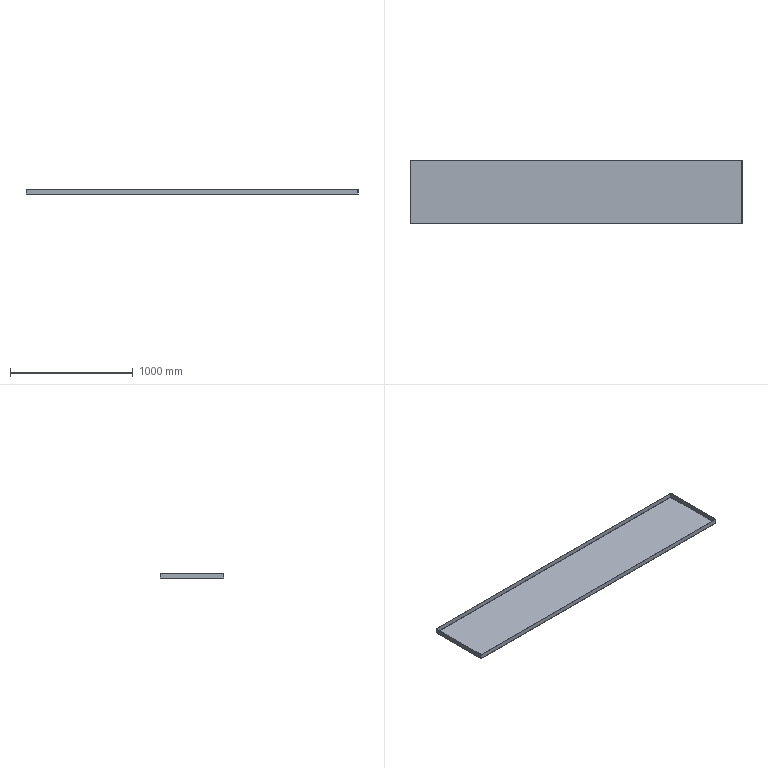Part | SolidWorks | features EdgeFlange 1, FlatPattern 1, SMBaseFlange 1, SheetMetal 1 | 1 solid | 38 faces | box 2700 x 518 x 40 mm | volume 3275069 mm3 | plane 22 | spline 8 | cylinder 8 | commonest cylinder face diameters 1.473 x4 5.473 x4
STEP:
#1=CARTESIAN_POINT('',(1347.263,256.263,-2.));
#2=VERTEX_POINT('',#1);
#3=CARTESIAN_POINT('',(1347.263,-256.263,-2.));
#4=VERTEX_POINT('',#3);
#5=CARTESIAN_POINT('',(1347.263,256.293,-2.));
#6=DIRECTION('',(0.,-1.,0.));
#7=VECTOR('',#6,1000.);
#8=LINE('',#5,#7);
#9=EDGE_CURVE('',#2,#4,#8,.T.);
#10=ORIENTED_EDGE('',*,*,#9,.T.);
#11=CARTESIAN_POINT('',(-1347.263,-256.263,-2.));
#12=VERTEX_POINT('',#11);
#13=CARTESIAN_POINT('',(1347.293,-256.263,-2.));
#14=DIRECTION('',(-1.,0.,0.));
#15=VECTOR('',#14,1000.);
#16=LINE('',#13,#15);
#17=EDGE_CURVE('',#4,#12,#16,.T.);
#18=ORIENTED_EDGE('',*,*,#17,.T.);
#19=CARTESIAN_POINT('',(-1347.263,256.263,-2.));
#20=VERTEX_POINT('',#19);
#21=CARTESIAN_POINT('',(-1347.263,-256.293,-2.));
#22=DIRECTION('',(0.,1.,0.));
#23=VECTOR('',#22,1000.);
#24=LINE('',#21,#23);
#25=EDGE_CURVE('',#12,#20,#24,.T.);
#26=ORIENTED_EDGE('',*,*,#25,.T.);
#27=CARTESIAN_POINT('',(-1347.293,256.263,-2.));
#28=DIRECTION('',(1.,0.,0.));
#29=VECTOR('',#28,1000.);
#30=LINE('',#27,#29);
#31=EDGE_CURVE('',#20,#2,#30,.T.);
#32=ORIENTED_EDGE('',*,*,#31,.T.);
#33=EDGE_LOOP('',(#10,#18,#26,#32));
#34=FACE_OUTER_BOUND('',#33,.T.);
#35=CARTESIAN_POINT('',(0.,0.,-2.));
#36=DIRECTION('',(0.,0.,-1.));
#37=DIRECTION('',(-1.,0.,0.));
#38=AXIS2_PLACEMENT_3D('',#35,#36,#37);
#39=PLANE('',#38);
#40=ADVANCED_FACE('',(#34),#39,.T.);
#41=CARTESIAN_POINT('',(1347.263,-256.263,0.));
#42=VERTEX_POINT('',#41);
#43=CARTESIAN_POINT('',(-1347.263,-256.263,0.));
#44=VERTEX_POINT('',#43);
#45=CARTESIAN_POINT('',(1347.293,-256.263,0.));
#46=DIRECTION('',(-1.,0.,0.));
#47=VECTOR('',#46,1000.);
#48=LINE('',#45,#47);
#49=EDGE_CURVE('',#42,#44,#48,.T.);
#50=ORIENTED_EDGE('',*,*,#49,.F.);
#51=CARTESIAN_POINT('',(1347.263,256.263,0.));
#52=VERTEX_POINT('',#51);
#53=CARTESIAN_POINT('',(1347.263,256.293,0.));
#54=DIRECTION('',(0.,-1.,0.));
#55=VECTOR('',#54,1000.);
#56=LINE('',#53,#55);
#57=EDGE_CURVE('',#52,#42,#56,.T.);
#58=ORIENTED_EDGE('',*,*,#57,.F.);
#59=CARTESIAN_POINT('',(-1347.263,256.263,0.));
#60=VERTEX_POINT('',#59);
#61=CARTESIAN_POINT('',(-1347.293,256.263,0.));
#62=DIRECTION('',(1.,0.,0.));
#63=VECTOR('',#62,1000.);
#64=LINE('',#61,#63);
#65=EDGE_CURVE('',#60,#52,#64,.T.);
#66=ORIENTED_EDGE('',*,*,#65,.F.);
#67=CARTESIAN_POINT('',(-1347.263,-256.293,0.));
#68=DIRECTION('',(0.,1.,0.));
#69=VECTOR('',#68,1000.);
#70=LINE('',#67,#69);
#71=EDGE_CURVE('',#44,#60,#70,.T.);
#72=ORIENTED_EDGE('',*,*,#71,.F.);
#73=EDGE_LOOP('',(#50,#58,#66,#72));
#74=FACE_OUTER_BOUND('',#73,.T.);
#75=CARTESIAN_POINT('',(0.,0.,0.));
#76=DIRECTION('',(0.,0.,-1.));
#77=DIRECTION('',(-1.,0.,0.));
#78=AXIS2_PLACEMENT_3D('',#75,#76,#77);
#79=PLANE('',#78);
#80=ADVANCED_FACE('',(#74),#79,.F.);
#81=CARTESIAN_POINT('',(1347.293,259.,0.7366));
#82=VERTEX_POINT('',#81);
#83=CARTESIAN_POINT('',(1347.293,257.,0.7366));
#84=VERTEX_POINT('',#83);
#85=CARTESIAN_POINT('',(1347.293,257.,0.7366));
#86=DIRECTION('',(0.,-1.,0.));
#87=VECTOR('',#86,1000.);
#88=LINE('',#85,#87);
#89=EDGE_CURVE('',#82,#84,#88,.T.);
#90=ORIENTED_EDGE('',*,*,#89,.T.);
#91=CARTESIAN_POINT('',(1347.263,256.263,0.));
#92=CARTESIAN_POINT('',(1347.268,256.456,0.));
#93=CARTESIAN_POINT('',(1347.273,256.648,0.07939));
#94=CARTESIAN_POINT('',(1347.283,256.921,0.3521));
#95=CARTESIAN_POINT('',(1347.288,257.,0.5438));
#96=CARTESIAN_POINT('',(1347.293,257.,0.7366));
#97=B_SPLINE_CURVE_WITH_KNOTS('',3,(#91,#92,#93,#94,#95,#96),.UNSPECIFIED.,.F.,.F.,(4,2,4),(0.,0.5,1.),.UNSPECIFIED.);
#98=EDGE_CURVE('',#52,#84,#97,.T.);
#99=ORIENTED_EDGE('',*,*,#98,.F.);
#100=CARTESIAN_POINT('',(1347.263,256.263,0.));
#101=DIRECTION('',(0.,0.,-1.));
#102=VECTOR('',#101,1000.);
#103=LINE('',#100,#102);
#104=EDGE_CURVE('',#52,#2,#103,.T.);
#105=ORIENTED_EDGE('',*,*,#104,.T.);
#106=CARTESIAN_POINT('',(1347.263,256.263,-2.));
#107=CARTESIAN_POINT('',(1347.266,256.622,-2.));
#108=CARTESIAN_POINT('',(1347.268,256.98,-1.929));
#109=CARTESIAN_POINT('',(1347.273,257.642,-1.655));
#110=CARTESIAN_POINT('',(1347.276,257.945,-1.452));
#111=CARTESIAN_POINT('',(1347.281,258.452,-0.9452));
#112=CARTESIAN_POINT('',(1347.283,258.655,-0.6416));
#113=CARTESIAN_POINT('',(1347.288,258.929,0.0203));
#114=CARTESIAN_POINT('',(1347.29,259.,0.3784));
#115=CARTESIAN_POINT('',(1347.293,259.,0.7366));
#116=B_SPLINE_CURVE_WITH_KNOTS('',3,(#106,#107,#108,#109,#110,#111,#112,#113,#114,#115),.UNSPECIFIED.,.F.,.F.,(4,2,2,2,4),(0.,0.25,0.5,0.75,1.),.UNSPECIFIED.);
#117=EDGE_CURVE('',#2,#82,#116,.T.);
#118=ORIENTED_EDGE('',*,*,#117,.T.);
#119=EDGE_LOOP('',(#90,#99,#105,#118));
#120=FACE_OUTER_BOUND('',#119,.T.);
#121=CARTESIAN_POINT('',(1347.263,256.263,-2.02));
#122=CARTESIAN_POINT('',(1347.266,256.624,-2.02));
#123=CARTESIAN_POINT('',(1347.268,256.985,-1.948));
#124=CARTESIAN_POINT('',(1347.273,257.652,-1.672));
#125=CARTESIAN_POINT('',(1347.276,257.957,-1.468));
#126=CARTESIAN_POINT('',(1347.281,258.468,-0.9575));
#127=CARTESIAN_POINT('',(1347.283,258.672,-0.6517));
#128=CARTESIAN_POINT('',(1347.288,258.948,0.01507));
#129=CARTESIAN_POINT('',(1347.29,259.02,0.3757));
#130=CARTESIAN_POINT('',(1347.293,259.02,0.7366));
#131=CARTESIAN_POINT('',(1347.263,256.263,-2.));
#132=CARTESIAN_POINT('',(1347.266,256.622,-2.));
#133=CARTESIAN_POINT('',(1347.268,256.98,-1.929));
#134=CARTESIAN_POINT('',(1347.273,257.642,-1.655));
#135=CARTESIAN_POINT('',(1347.276,257.945,-1.452));
#136=CARTESIAN_POINT('',(1347.281,258.452,-0.9452));
#137=CARTESIAN_POINT('',(1347.283,258.655,-0.6416));
#138=CARTESIAN_POINT('',(1347.288,258.929,0.0203));
#139=CARTESIAN_POINT('',(1347.29,259.,0.3783));
#140=CARTESIAN_POINT('',(1347.293,259.,0.7366));
#141=CARTESIAN_POINT('',(1347.263,256.263,0.));
#142=CARTESIAN_POINT('',(1347.266,256.36,0.));
#143=CARTESIAN_POINT('',(1347.268,256.456,0.01917));
#144=CARTESIAN_POINT('',(1347.273,256.634,0.09297));
#145=CARTESIAN_POINT('',(1347.276,256.716,0.1476));
#146=CARTESIAN_POINT('',(1347.281,256.852,0.2839));
#147=CARTESIAN_POINT('',(1347.283,256.907,0.3656));
#148=CARTESIAN_POINT('',(1347.288,256.981,0.5438));
#149=CARTESIAN_POINT('',(1347.29,257.,0.6402));
#150=CARTESIAN_POINT('',(1347.293,257.,0.7366));
#151=CARTESIAN_POINT('',(1347.263,256.263,0.0202));
#152=CARTESIAN_POINT('',(1347.266,256.357,0.0202));
#153=CARTESIAN_POINT('',(1347.268,256.451,0.03885));
#154=CARTESIAN_POINT('',(1347.273,256.624,0.1106));
#155=CARTESIAN_POINT('',(1347.276,256.704,0.1637));
#156=CARTESIAN_POINT('',(1347.281,256.836,0.2963));
#157=CARTESIAN_POINT('',(1347.283,256.889,0.3758));
#158=CARTESIAN_POINT('',(1347.288,256.961,0.5491));
#159=CARTESIAN_POINT('',(1347.29,256.98,0.6428));
#160=CARTESIAN_POINT('',(1347.293,256.98,0.7366));
#161=B_SPLINE_SURFACE_WITH_KNOTS('',1,3,((#121,#122,#123,#124,#125,#126,#127,#128,#129,#130),(#131,#132,#133,#134,#135,#136,#137,#138,#139,#140),(#141,#142,#143,#144,#145,#146,#147,#148,#149,#150),(#151,#152,#153,#154,#155,#156,#157,#158,#159,#160)),.UNSPECIFIED.,.F.,.F.,.F.,(2,1,1,2),(4,2,2,2,4),(-0.01,0.,1.,1.01),(0.,0.25,0.5,0.75,1.),.UNSPECIFIED.);
#162=ADVANCED_FACE('',(#120),#161,.F.);
#163=CARTESIAN_POINT('',(-1347.293,257.,0.7366));
#164=VERTEX_POINT('',#163);
#165=CARTESIAN_POINT('',(-1347.293,257.,0.7366));
#166=CARTESIAN_POINT('',(-1347.288,257.,0.5438));
#167=CARTESIAN_POINT('',(-1347.283,256.921,0.3521));
#168=CARTESIAN_POINT('',(-1347.273,256.648,0.07939));
#169=CARTESIAN_POINT('',(-1347.268,256.456,0.));
#170=CARTESIAN_POINT('',(-1347.263,256.263,0.));
#171=B_SPLINE_CURVE_WITH_KNOTS('',3,(#165,#166,#167,#168,#169,#170),.UNSPECIFIED.,.F.,.F.,(4,2,4),(0.,0.5,1.),.UNSPECIFIED.);
#172=EDGE_CURVE('',#164,#60,#171,.T.);
#173=ORIENTED_EDGE('',*,*,#172,.F.);
#174=CARTESIAN_POINT('',(-1347.293,259.,0.7366));
#175=VERTEX_POINT('',#174);
#176=CARTESIAN_POINT('',(-1347.293,257.,0.7366));
#177=DIRECTION('',(0.,-1.,0.));
#178=VECTOR('',#177,1000.);
#179=LINE('',#176,#178);
#180=EDGE_CURVE('',#175,#164,#179,.T.);
#181=ORIENTED_EDGE('',*,*,#180,.F.);
#182=CARTESIAN_POINT('',(-1347.293,259.,0.7366));
#183=CARTESIAN_POINT('',(-1347.29,259.,0.3784));
#184=CARTESIAN_POINT('',(-1347.288,258.929,0.0203));
#185=CARTESIAN_POINT('',(-1347.283,258.655,-0.6416));
#186=CARTESIAN_POINT('',(-1347.281,258.452,-0.9452));
#187=CARTESIAN_POINT('',(-1347.276,257.945,-1.452));
#188=CARTESIAN_POINT('',(-1347.273,257.642,-1.655));
#189=CARTESIAN_POINT('',(-1347.268,256.98,-1.929));
#190=CARTESIAN_POINT('',(-1347.266,256.622,-2.));
#191=CARTESIAN_POINT('',(-1347.263,256.263,-2.));
#192=B_SPLINE_CURVE_WITH_KNOTS('',3,(#182,#183,#184,#185,#186,#187,#188,#189,#190,#191),.UNSPECIFIED.,.F.,.F.,(4,2,2,2,4),(0.,0.25,0.5,0.75,1.),.UNSPECIFIED.);
#193=EDGE_CURVE('',#175,#20,#192,.T.);
#194=ORIENTED_EDGE('',*,*,#193,.T.);
#195=CARTESIAN_POINT('',(-1347.263,256.263,0.));
#196=DIRECTION('',(0.,0.,-1.));
#197=VECTOR('',#196,1000.);
#198=LINE('',#195,#197);
#199=EDGE_CURVE('',#60,#20,#198,.T.);
#200=ORIENTED_EDGE('',*,*,#199,.F.);
#201=EDGE_LOOP('',(#173,#181,#194,#200));
#202=FACE_OUTER_BOUND('',#201,.T.);
#203=CARTESIAN_POINT('',(-1347.293,259.02,0.7366));
#204=CARTESIAN_POINT('',(-1347.29,259.02,0.3757));
#205=CARTESIAN_POINT('',(-1347.288,258.948,0.01507));
#206=CARTESIAN_POINT('',(-1347.283,258.672,-0.6517));
#207=CARTESIAN_POINT('',(-1347.281,258.468,-0.9575));
#208=CARTESIAN_POINT('',(-1347.276,257.957,-1.468));
#209=CARTESIAN_POINT('',(-1347.273,257.652,-1.672));
#210=CARTESIAN_POINT('',(-1347.268,256.985,-1.948));
#211=CARTESIAN_POINT('',(-1347.266,256.624,-2.02));
#212=CARTESIAN_POINT('',(-1347.263,256.263,-2.02));
#213=CARTESIAN_POINT('',(-1347.293,259.,0.7366));
#214=CARTESIAN_POINT('',(-1347.29,259.,0.3783));
#215=CARTESIAN_POINT('',(-1347.288,258.929,0.0203));
#216=CARTESIAN_POINT('',(-1347.283,258.655,-0.6416));
#217=CARTESIAN_POINT('',(-1347.281,258.452,-0.9452));
#218=CARTESIAN_POINT('',(-1347.276,257.945,-1.452));
#219=CARTESIAN_POINT('',(-1347.273,257.642,-1.655));
#220=CARTESIAN_POINT('',(-1347.268,256.98,-1.929));
#221=CARTESIAN_POINT('',(-1347.266,256.622,-2.));
#222=CARTESIAN_POINT('',(-1347.263,256.263,-2.));
#223=CARTESIAN_POINT('',(-1347.293,257.,0.7366));
#224=CARTESIAN_POINT('',(-1347.29,257.,0.6402));
#225=CARTESIAN_POINT('',(-1347.288,256.981,0.5438));
#226=CARTESIAN_POINT('',(-1347.283,256.907,0.3656));
#227=CARTESIAN_POINT('',(-1347.281,256.852,0.2839));
#228=CARTESIAN_POINT('',(-1347.276,256.716,0.1476));
#229=CARTESIAN_POINT('',(-1347.273,256.634,0.09297));
#230=CARTESIAN_POINT('',(-1347.268,256.456,0.01917));
#231=CARTESIAN_POINT('',(-1347.266,256.36,0.));
#232=CARTESIAN_POINT('',(-1347.263,256.263,0.));
#233=CARTESIAN_POINT('',(-1347.293,256.98,0.7366));
#234=CARTESIAN_POINT('',(-1347.29,256.98,0.6428));
#235=CARTESIAN_POINT('',(-1347.288,256.961,0.5491));
#236=CARTESIAN_POINT('',(-1347.283,256.889,0.3758));
#237=CARTESIAN_POINT('',(-1347.281,256.836,0.2963));
#238=CARTESIAN_POINT('',(-1347.276,256.704,0.1637));
#239=CARTESIAN_POINT('',(-1347.273,256.624,0.1106));
#240=CARTESIAN_POINT('',(-1347.268,256.451,0.03885));
#241=CARTESIAN_POINT('',(-1347.266,256.357,0.0202));
#242=CARTESIAN_POINT('',(-1347.263,256.263,0.0202));
#243=B_SPLINE_SURFACE_WITH_KNOTS('',1,3,((#203,#204,#205,#206,#207,#208,#209,#210,#211,#212),(#213,#214,#215,#216,#217,#218,#219,#220,#221,#222),(#223,#224,#225,#226,#227,#228,#229,#230,#231,#232),(#233,#234,#235,#236,#237,#238,#239,#240,#241,#242)),.UNSPECIFIED.,.F.,.F.,.F.,(2,1,1,2),(4,2,2,2,4),(-0.01,0.,1.,1.01),(0.,0.25,0.5,0.75,1.),.UNSPECIFIED.);
#244=ADVANCED_FACE('',(#202),#243,.F.);
#245=ORIENTED_EDGE('',*,*,#31,.F.);
#246=ORIENTED_EDGE('',*,*,#193,.F.);
#247=CARTESIAN_POINT('',(0.,259.,0.7366));
#248=DIRECTION('',(-1.,0.,0.));
#249=VECTOR('',#248,1000.);
#250=LINE('',#247,#249);
#251=EDGE_CURVE('',#82,#175,#250,.T.);
#252=ORIENTED_EDGE('',*,*,#251,.F.);
#253=ORIENTED_EDGE('',*,*,#117,.F.);
#254=EDGE_LOOP('',(#245,#246,#252,#253));
#255=FACE_OUTER_BOUND('',#254,.T.);
#256=CARTESIAN_POINT('',(-1347.293,256.263,0.7366));
#257=DIRECTION('',(-1.,0.,0.));
#258=DIRECTION('',(0.,1.,0.));
#259=AXIS2_PLACEMENT_3D('',#256,#257,#258);
#260=CYLINDRICAL_SURFACE('',#259,2.737);
#261=ADVANCED_FACE('',(#255),#260,.T.);
#262=ORIENTED_EDGE('',*,*,#65,.T.);
#263=ORIENTED_EDGE('',*,*,#98,.T.);
#264=CARTESIAN_POINT('',(1350.,257.,0.7366));
#265=DIRECTION('',(-1.,0.,0.));
#266=VECTOR('',#265,1000.);
#267=LINE('',#264,#266);
#268=EDGE_CURVE('',#84,#164,#267,.T.);
#269=ORIENTED_EDGE('',*,*,#268,.T.);
#270=ORIENTED_EDGE('',*,*,#172,.T.);
#271=EDGE_LOOP('',(#262,#263,#269,#270));
#272=FACE_OUTER_BOUND('',#271,.T.);
#273=CARTESIAN_POINT('',(-1347.293,256.263,0.7366));
#274=DIRECTION('',(-1.,0.,0.));
#275=DIRECTION('',(0.,1.,0.));
#276=AXIS2_PLACEMENT_3D('',#273,#274,#275);
#277=CYLINDRICAL_SURFACE('',#276,0.7366);
#278=ADVANCED_FACE('',(#272),#277,.F.);
#279=CARTESIAN_POINT('',(1347.293,257.,38.));
#280=VERTEX_POINT('',#279);
#281=CARTESIAN_POINT('',(1347.293,259.,38.));
#282=VERTEX_POINT('',#281);
#283=CARTESIAN_POINT('',(1347.293,259.,38.));
#284=DIRECTION('',(0.,1.,0.));
#285=VECTOR('',#284,1000.);
#286=LINE('',#283,#285);
#287=EDGE_CURVE('',#280,#282,#286,.T.);
#288=ORIENTED_EDGE('',*,*,#287,.F.);
#289=CARTESIAN_POINT('',(1347.293,257.,0.));
#290=DIRECTION('',(0.,0.,1.));
#291=VECTOR('',#290,1000.);
#292=LINE('',#289,#291);
#293=EDGE_CURVE('',#84,#280,#292,.T.);
#294=ORIENTED_EDGE('',*,*,#293,.F.);
#295=ORIENTED_EDGE('',*,*,#89,.F.);
#296=CARTESIAN_POINT('',(1347.293,259.,0.));
#297=DIRECTION('',(0.,0.,-1.));
#298=VECTOR('',#297,1000.);
#299=LINE('',#296,#298);
#300=EDGE_CURVE('',#282,#82,#299,.T.);
#301=ORIENTED_EDGE('',*,*,#300,.F.);
#302=EDGE_LOOP('',(#288,#294,#295,#301));
#303=FACE_OUTER_BOUND('',#302,.T.);
#304=CARTESIAN_POINT('',(1347.293,257.,0.));
#305=DIRECTION('',(1.,0.,0.));
#306=DIRECTION('',(0.,0.,-1.));
#307=AXIS2_PLACEMENT_3D('',#304,#305,#306);
#308=PLANE('',#307);
#309=ADVANCED_FACE('',(#303),#308,.T.);
#310=CARTESIAN_POINT('',(-1347.293,259.,38.));
#311=VERTEX_POINT('',#310);
#312=CARTESIAN_POINT('',(-1347.293,259.,0.));
#313=DIRECTION('',(0.,0.,-1.));
#314=VECTOR('',#313,1000.);
#315=LINE('',#312,#314);
#316=EDGE_CURVE('',#311,#175,#315,.T.);
#317=ORIENTED_EDGE('',*,*,#316,.F.);
#318=CARTESIAN_POINT('',(-1350.,259.,38.));
#319=DIRECTION('',(-1.,0.,0.));
#320=VECTOR('',#319,1000.);
#321=LINE('',#318,#320);
#322=EDGE_CURVE('',#282,#311,#321,.T.);
#323=ORIENTED_EDGE('',*,*,#322,.F.);
#324=ORIENTED_EDGE('',*,*,#300,.T.);
#325=ORIENTED_EDGE('',*,*,#251,.T.);
#326=EDGE_LOOP('',(#317,#323,#324,#325));
#327=FACE_OUTER_BOUND('',#326,.T.);
#328=CARTESIAN_POINT('',(0.,259.,0.));
#329=DIRECTION('',(0.,1.,0.));
#330=DIRECTION('',(0.,0.,1.));
#331=AXIS2_PLACEMENT_3D('',#328,#329,#330);
#332=PLANE('',#331);
#333=ADVANCED_FACE('',(#327),#332,.T.);
#334=CARTESIAN_POINT('',(-1347.293,257.,38.));
#335=VERTEX_POINT('',#334);
#336=CARTESIAN_POINT('',(0.,257.,38.));
#337=DIRECTION('',(-1.,0.,0.));
#338=VECTOR('',#337,1000.);
#339=LINE('',#336,#338);
#340=EDGE_CURVE('',#280,#335,#339,.T.);
#341=ORIENTED_EDGE('',*,*,#340,.T.);
#342=CARTESIAN_POINT('',(-1347.293,257.,0.));
#343=DIRECTION('',(0.,0.,1.));
#344=VECTOR('',#343,1000.);
#345=LINE('',#342,#344);
#346=EDGE_CURVE('',#164,#335,#345,.T.);
#347=ORIENTED_EDGE('',*,*,#346,.F.);
#348=ORIENTED_EDGE('',*,*,#268,.F.);
#349=ORIENTED_EDGE('',*,*,#293,.T.);
#350=EDGE_LOOP('',(#341,#347,#348,#349));
#351=FACE_OUTER_BOUND('',#350,.T.);
#352=CARTESIAN_POINT('',(0.,257.,0.));
#353=DIRECTION('',(0.,1.,0.));
#354=DIRECTION('',(0.,0.,1.));
#355=AXIS2_PLACEMENT_3D('',#352,#353,#354);
#356=PLANE('',#355);
#357=ADVANCED_FACE('',(#351),#356,.F.);
#358=CARTESIAN_POINT('',(-1347.293,257.,38.));
#359=DIRECTION('',(0.,1.,0.));
#360=VECTOR('',#359,1000.);
#361=LINE('',#358,#360);
#362=EDGE_CURVE('',#335,#311,#361,.T.);
#363=ORIENTED_EDGE('',*,*,#362,.F.);
#364=ORIENTED_EDGE('',*,*,#340,.F.);
#365=ORIENTED_EDGE('',*,*,#287,.T.);
#366=ORIENTED_EDGE('',*,*,#322,.T.);
#367=EDGE_LOOP('',(#363,#364,#365,#366));
#368=FACE_OUTER_BOUND('',#367,.T.);
#369=CARTESIAN_POINT('',(-1350.,259.,38.));
#370=DIRECTION('',(0.,0.,1.));
#371=DIRECTION('',(0.,-1.,0.));
#372=AXIS2_PLACEMENT_3D('',#369,#370,#371);
#373=PLANE('',#372);
#374=ADVANCED_FACE('',(#368),#373,.T.);
#375=ORIENTED_EDGE('',*,*,#346,.T.);
#376=ORIENTED_EDGE('',*,*,#362,.T.);
#377=ORIENTED_EDGE('',*,*,#316,.T.);
#378=ORIENTED_EDGE('',*,*,#180,.T.);
#379=EDGE_LOOP('',(#375,#376,#377,#378));
#380=FACE_OUTER_BOUND('',#379,.T.);
#381=CARTESIAN_POINT('',(-1347.293,257.,0.));
#382=DIRECTION('',(1.,0.,0.));
#383=DIRECTION('',(0.,0.,-1.));
#384=AXIS2_PLACEMENT_3D('',#381,#382,#383);
#385=PLANE('',#384);
#386=ADVANCED_FACE('',(#380),#385,.F.);
#387=CARTESIAN_POINT('',(-1350.,256.293,0.7366));
#388=VERTEX_POINT('',#387);
#389=CARTESIAN_POINT('',(-1348.,256.293,0.7366));
#390=VERTEX_POINT('',#389);
#391=CARTESIAN_POINT('',(-1348.,256.293,0.7366));
#392=DIRECTION('',(1.,0.,0.));
#393=VECTOR('',#392,1000.);
#394=LINE('',#391,#393);
#395=EDGE_CURVE('',#388,#390,#394,.T.);
#396=ORIENTED_EDGE('',*,*,#395,.T.);
#397=CARTESIAN_POINT('',(-1347.263,256.263,0.));
#398=CARTESIAN_POINT('',(-1347.456,256.268,0.));
#399=CARTESIAN_POINT('',(-1347.648,256.273,0.07939));
#400=CARTESIAN_POINT('',(-1347.921,256.283,0.3521));
#401=CARTESIAN_POINT('',(-1348.,256.288,0.5438));
#402=CARTESIAN_POINT('',(-1348.,256.293,0.7366));
#403=B_SPLINE_CURVE_WITH_KNOTS('',3,(#397,#398,#399,#400,#401,#402),.UNSPECIFIED.,.F.,.F.,(4,2,4),(0.,0.5,1.),.UNSPECIFIED.);
#404=EDGE_CURVE('',#60,#390,#403,.T.);
#405=ORIENTED_EDGE('',*,*,#404,.F.);
#406=ORIENTED_EDGE('',*,*,#199,.T.);
#407=CARTESIAN_POINT('',(-1347.263,256.263,-2.));
#408=CARTESIAN_POINT('',(-1347.622,256.266,-2.));
#409=CARTESIAN_POINT('',(-1347.98,256.268,-1.929));
#410=CARTESIAN_POINT('',(-1348.642,256.273,-1.655));
#411=CARTESIAN_POINT('',(-1348.945,256.276,-1.452));
#412=CARTESIAN_POINT('',(-1349.452,256.281,-0.9452));
#413=CARTESIAN_POINT('',(-1349.655,256.283,-0.6416));
#414=CARTESIAN_POINT('',(-1349.929,256.288,0.0203));
#415=CARTESIAN_POINT('',(-1350.,256.29,0.3784));
#416=CARTESIAN_POINT('',(-1350.,256.293,0.7366));
#417=B_SPLINE_CURVE_WITH_KNOTS('',3,(#407,#408,#409,#410,#411,#412,#413,#414,#415,#416),.UNSPECIFIED.,.F.,.F.,(4,2,2,2,4),(0.,0.25,0.5,0.75,1.),.UNSPECIFIED.);
#418=EDGE_CURVE('',#20,#388,#417,.T.);
#419=ORIENTED_EDGE('',*,*,#418,.T.);
#420=EDGE_LOOP('',(#396,#405,#406,#419));
#421=FACE_OUTER_BOUND('',#420,.T.);
#422=CARTESIAN_POINT('',(-1347.263,256.263,-2.02));
#423=CARTESIAN_POINT('',(-1347.624,256.266,-2.02));
#424=CARTESIAN_POINT('',(-1347.985,256.268,-1.948));
#425=CARTESIAN_POINT('',(-1348.652,256.273,-1.672));
#426=CARTESIAN_POINT('',(-1348.957,256.276,-1.468));
#427=CARTESIAN_POINT('',(-1349.468,256.281,-0.9575));
#428=CARTESIAN_POINT('',(-1349.672,256.283,-0.6517));
#429=CARTESIAN_POINT('',(-1349.948,256.288,0.01507));
#430=CARTESIAN_POINT('',(-1350.02,256.29,0.3757));
#431=CARTESIAN_POINT('',(-1350.02,256.293,0.7366));
#432=CARTESIAN_POINT('',(-1347.263,256.263,-2.));
#433=CARTESIAN_POINT('',(-1347.622,256.266,-2.));
#434=CARTESIAN_POINT('',(-1347.98,256.268,-1.929));
#435=CARTESIAN_POINT('',(-1348.642,256.273,-1.655));
#436=CARTESIAN_POINT('',(-1348.945,256.276,-1.452));
#437=CARTESIAN_POINT('',(-1349.452,256.281,-0.9452));
#438=CARTESIAN_POINT('',(-1349.655,256.283,-0.6416));
#439=CARTESIAN_POINT('',(-1349.929,256.288,0.0203));
#440=CARTESIAN_POINT('',(-1350.,256.29,0.3783));
#441=CARTESIAN_POINT('',(-1350.,256.293,0.7366));
#442=CARTESIAN_POINT('',(-1347.263,256.263,0.));
#443=CARTESIAN_POINT('',(-1347.36,256.266,0.));
#444=CARTESIAN_POINT('',(-1347.456,256.268,0.01917));
#445=CARTESIAN_POINT('',(-1347.634,256.273,0.09297));
#446=CARTESIAN_POINT('',(-1347.716,256.276,0.1476));
#447=CARTESIAN_POINT('',(-1347.852,256.281,0.2839));
#448=CARTESIAN_POINT('',(-1347.907,256.283,0.3656));
#449=CARTESIAN_POINT('',(-1347.981,256.288,0.5438));
#450=CARTESIAN_POINT('',(-1348.,256.29,0.6402));
#451=CARTESIAN_POINT('',(-1348.,256.293,0.7366));
#452=CARTESIAN_POINT('',(-1347.263,256.263,0.0202));
#453=CARTESIAN_POINT('',(-1347.357,256.266,0.0202));
#454=CARTESIAN_POINT('',(-1347.451,256.268,0.03885));
#455=CARTESIAN_POINT('',(-1347.624,256.273,0.1106));
#456=CARTESIAN_POINT('',(-1347.704,256.276,0.1637));
#457=CARTESIAN_POINT('',(-1347.836,256.281,0.2963));
#458=CARTESIAN_POINT('',(-1347.889,256.283,0.3758));
#459=CARTESIAN_POINT('',(-1347.961,256.288,0.5491));
#460=CARTESIAN_POINT('',(-1347.98,256.29,0.6428));
#461=CARTESIAN_POINT('',(-1347.98,256.293,0.7366));
#462=B_SPLINE_SURFACE_WITH_KNOTS('',1,3,((#422,#423,#424,#425,#426,#427,#428,#429,#430,#431),(#432,#433,#434,#435,#436,#437,#438,#439,#440,#441),(#442,#443,#444,#445,#446,#447,#448,#449,#450,#451),(#452,#453,#454,#455,#456,#457,#458,#459,#460,#461)),.UNSPECIFIED.,.F.,.F.,.F.,(2,1,1,2),(4,2,2,2,4),(-0.01,0.,1.,1.01),(0.,0.25,0.5,0.75,1.),.UNSPECIFIED.);
#463=ADVANCED_FACE('',(#421),#462,.F.);
#464=CARTESIAN_POINT('',(-1348.,-256.293,0.7366));
#465=VERTEX_POINT('',#464);
#466=CARTESIAN_POINT('',(-1348.,-256.293,0.7366));
#467=CARTESIAN_POINT('',(-1348.,-256.288,0.5438));
#468=CARTESIAN_POINT('',(-1347.921,-256.283,0.3521));
#469=CARTESIAN_POINT('',(-1347.648,-256.273,0.07939));
#470=CARTESIAN_POINT('',(-1347.456,-256.268,0.));
#471=CARTESIAN_POINT('',(-1347.263,-256.263,0.));
#472=B_SPLINE_CURVE_WITH_KNOTS('',3,(#466,#467,#468,#469,#470,#471),.UNSPECIFIED.,.F.,.F.,(4,2,4),(0.,0.5,1.),.UNSPECIFIED.);
#473=EDGE_CURVE('',#465,#44,#472,.T.);
#474=ORIENTED_EDGE('',*,*,#473,.F.);
#475=CARTESIAN_POINT('',(-1350.,-256.293,0.7366));
#476=VERTEX_POINT('',#475);
#477=CARTESIAN_POINT('',(-1348.,-256.293,0.7366));
#478=DIRECTION('',(1.,0.,0.));
#479=VECTOR('',#478,1000.);
#480=LINE('',#477,#479);
#481=EDGE_CURVE('',#476,#465,#480,.T.);
#482=ORIENTED_EDGE('',*,*,#481,.F.);
#483=CARTESIAN_POINT('',(-1350.,-256.293,0.7366));
#484=CARTESIAN_POINT('',(-1350.,-256.29,0.3784));
#485=CARTESIAN_POINT('',(-1349.929,-256.288,0.0203));
#486=CARTESIAN_POINT('',(-1349.655,-256.283,-0.6416));
#487=CARTESIAN_POINT('',(-1349.452,-256.281,-0.9452));
#488=CARTESIAN_POINT('',(-1348.945,-256.276,-1.452));
#489=CARTESIAN_POINT('',(-1348.642,-256.273,-1.655));
#490=CARTESIAN_POINT('',(-1347.98,-256.268,-1.929));
#491=CARTESIAN_POINT('',(-1347.622,-256.266,-2.));
#492=CARTESIAN_POINT('',(-1347.263,-256.263,-2.));
#493=B_SPLINE_CURVE_WITH_KNOTS('',3,(#483,#484,#485,#486,#487,#488,#489,#490,#491,#492),.UNSPECIFIED.,.F.,.F.,(4,2,2,2,4),(0.,0.25,0.5,0.75,1.),.UNSPECIFIED.);
#494=EDGE_CURVE('',#476,#12,#493,.T.);
#495=ORIENTED_EDGE('',*,*,#494,.T.);
#496=CARTESIAN_POINT('',(-1347.263,-256.263,0.));
#497=DIRECTION('',(0.,0.,-1.));
#498=VECTOR('',#497,1000.);
#499=LINE('',#496,#498);
#500=EDGE_CURVE('',#44,#12,#499,.T.);
#501=ORIENTED_EDGE('',*,*,#500,.F.);
#502=EDGE_LOOP('',(#474,#482,#495,#501));
#503=FACE_OUTER_BOUND('',#502,.T.);
#504=CARTESIAN_POINT('',(-1350.02,-256.293,0.7366));
#505=CARTESIAN_POINT('',(-1350.02,-256.29,0.3757));
#506=CARTESIAN_POINT('',(-1349.948,-256.288,0.01507));
#507=CARTESIAN_POINT('',(-1349.672,-256.283,-0.6517));
#508=CARTESIAN_POINT('',(-1349.468,-256.281,-0.9575));
#509=CARTESIAN_POINT('',(-1348.957,-256.276,-1.468));
#510=CARTESIAN_POINT('',(-1348.652,-256.273,-1.672));
#511=CARTESIAN_POINT('',(-1347.985,-256.268,-1.948));
#512=CARTESIAN_POINT('',(-1347.624,-256.266,-2.02));
#513=CARTESIAN_POINT('',(-1347.263,-256.263,-2.02));
#514=CARTESIAN_POINT('',(-1350.,-256.293,0.7366));
#515=CARTESIAN_POINT('',(-1350.,-256.29,0.3783));
#516=CARTESIAN_POINT('',(-1349.929,-256.288,0.0203));
#517=CARTESIAN_POINT('',(-1349.655,-256.283,-0.6416));
#518=CARTESIAN_POINT('',(-1349.452,-256.281,-0.9452));
#519=CARTESIAN_POINT('',(-1348.945,-256.276,-1.452));
#520=CARTESIAN_POINT('',(-1348.642,-256.273,-1.655));
#521=CARTESIAN_POINT('',(-1347.98,-256.268,-1.929));
#522=CARTESIAN_POINT('',(-1347.622,-256.266,-2.));
#523=CARTESIAN_POINT('',(-1347.263,-256.263,-2.));
#524=CARTESIAN_POINT('',(-1348.,-256.293,0.7366));
#525=CARTESIAN_POINT('',(-1348.,-256.29,0.6402));
#526=CARTESIAN_POINT('',(-1347.981,-256.288,0.5438));
#527=CARTESIAN_POINT('',(-1347.907,-256.283,0.3656));
#528=CARTESIAN_POINT('',(-1347.852,-256.281,0.2839));
#529=CARTESIAN_POINT('',(-1347.716,-256.276,0.1476));
#530=CARTESIAN_POINT('',(-1347.634,-256.273,0.09297));
#531=CARTESIAN_POINT('',(-1347.456,-256.268,0.01917));
#532=CARTESIAN_POINT('',(-1347.36,-256.266,0.));
#533=CARTESIAN_POINT('',(-1347.263,-256.263,0.));
#534=CARTESIAN_POINT('',(-1347.98,-256.293,0.7366));
#535=CARTESIAN_POINT('',(-1347.98,-256.29,0.6428));
#536=CARTESIAN_POINT('',(-1347.961,-256.288,0.5491));
#537=CARTESIAN_POINT('',(-1347.889,-256.283,0.3758));
#538=CARTESIAN_POINT('',(-1347.836,-256.281,0.2963));
#539=CARTESIAN_POINT('',(-1347.704,-256.276,0.1637));
#540=CARTESIAN_POINT('',(-1347.624,-256.273,0.1106));
#541=CARTESIAN_POINT('',(-1347.451,-256.268,0.03885));
#542=CARTESIAN_POINT('',(-1347.357,-256.266,0.0202));
#543=CARTESIAN_POINT('',(-1347.263,-256.263,0.0202));
#544=B_SPLINE_SURFACE_WITH_KNOTS('',1,3,((#504,#505,#506,#507,#508,#509,#510,#511,#512,#513),(#514,#515,#516,#517,#518,#519,#520,#521,#522,#523),(#524,#525,#526,#527,#528,#529,#530,#531,#532,#533),(#534,#535,#536,#537,#538,#539,#540,#541,#542,#543)),.UNSPECIFIED.,.F.,.F.,.F.,(2,1,1,2),(4,2,2,2,4),(-0.01,0.,1.,1.01),(0.,0.25,0.5,0.75,1.),.UNSPECIFIED.);
#545=ADVANCED_FACE('',(#503),#544,.F.);
#546=ORIENTED_EDGE('',*,*,#25,.F.);
#547=ORIENTED_EDGE('',*,*,#494,.F.);
#548=CARTESIAN_POINT('',(-1350.,259.,0.7366));
#549=DIRECTION('',(0.,1.,0.));
#550=VECTOR('',#549,1000.);
#551=LINE('',#548,#550);
#552=EDGE_CURVE('',#476,#388,#551,.T.);
#553=ORIENTED_EDGE('',*,*,#552,.T.);
#554=ORIENTED_EDGE('',*,*,#418,.F.);
#555=EDGE_LOOP('',(#546,#547,#553,#554));
#556=FACE_OUTER_BOUND('',#555,.T.);
#557=CARTESIAN_POINT('',(-1347.263,-256.293,0.7366));
#558=DIRECTION('',(0.,-1.,0.));
#559=DIRECTION('',(-1.,0.,0.));
#560=AXIS2_PLACEMENT_3D('',#557,#558,#559);
#561=CYLINDRICAL_SURFACE('',#560,2.737);
#562=ADVANCED_FACE('',(#556),#561,.T.);
#563=ORIENTED_EDGE('',*,*,#71,.T.);
#564=ORIENTED_EDGE('',*,*,#404,.T.);
#565=CARTESIAN_POINT('',(-1348.,259.,0.7366));
#566=DIRECTION('',(0.,-1.,0.));
#567=VECTOR('',#566,1000.);
#568=LINE('',#565,#567);
#569=EDGE_CURVE('',#390,#465,#568,.T.);
#570=ORIENTED_EDGE('',*,*,#569,.T.);
#571=ORIENTED_EDGE('',*,*,#473,.T.);
#572=EDGE_LOOP('',(#563,#564,#570,#571));
#573=FACE_OUTER_BOUND('',#572,.T.);
#574=CARTESIAN_POINT('',(-1347.263,-256.293,0.7366));
#575=DIRECTION('',(0.,-1.,0.));
#576=DIRECTION('',(-1.,0.,0.));
#577=AXIS2_PLACEMENT_3D('',#574,#575,#576);
#578=CYLINDRICAL_SURFACE('',#577,0.7366);
#579=ADVANCED_FACE('',(#573),#578,.F.);
#580=CARTESIAN_POINT('',(-1348.,256.293,38.));
#581=VERTEX_POINT('',#580);
#582=CARTESIAN_POINT('',(-1350.,256.293,38.));
#583=VERTEX_POINT('',#582);
#584=CARTESIAN_POINT('',(-1350.,256.293,38.));
#585=DIRECTION('',(-1.,0.,0.));
#586=VECTOR('',#585,1000.);
#587=LINE('',#584,#586);
#588=EDGE_CURVE('',#581,#583,#587,.T.);
#589=ORIENTED_EDGE('',*,*,#588,.F.);
#590=CARTESIAN_POINT('',(-1348.,256.293,0.));
#591=DIRECTION('',(0.,0.,1.));
#592=VECTOR('',#591,1000.);
#593=LINE('',#590,#592);
#594=EDGE_CURVE('',#390,#581,#593,.T.);
#595=ORIENTED_EDGE('',*,*,#594,.F.);
#596=ORIENTED_EDGE('',*,*,#395,.F.);
#597=CARTESIAN_POINT('',(-1350.,256.293,0.));
#598=DIRECTION('',(0.,0.,1.));
#599=VECTOR('',#598,1000.);
#600=LINE('',#597,#599);
#601=EDGE_CURVE('',#388,#583,#600,.T.);
#602=ORIENTED_EDGE('',*,*,#601,.T.);
#603=EDGE_LOOP('',(#589,#595,#596,#602));
#604=FACE_OUTER_BOUND('',#603,.T.);
#605=CARTESIAN_POINT('',(-1348.,256.293,0.));
#606=DIRECTION('',(0.,1.,0.));
#607=DIRECTION('',(0.,0.,1.));
#608=AXIS2_PLACEMENT_3D('',#605,#606,#607);
#609=PLANE('',#608);
#610=ADVANCED_FACE('',(#604),#609,.T.);
#611=ORIENTED_EDGE('',*,*,#552,.F.);
#612=CARTESIAN_POINT('',(-1350.,-256.293,38.));
#613=VERTEX_POINT('',#612);
#614=CARTESIAN_POINT('',(-1350.,-256.293,0.));
#615=DIRECTION('',(0.,0.,1.));
#616=VECTOR('',#615,1000.);
#617=LINE('',#614,#616);
#618=EDGE_CURVE('',#476,#613,#617,.T.);
#619=ORIENTED_EDGE('',*,*,#618,.T.);
#620=CARTESIAN_POINT('',(-1350.,259.,38.));
#621=DIRECTION('',(0.,-1.,0.));
#622=VECTOR('',#621,1000.);
#623=LINE('',#620,#622);
#624=EDGE_CURVE('',#583,#613,#623,.T.);
#625=ORIENTED_EDGE('',*,*,#624,.F.);
#626=ORIENTED_EDGE('',*,*,#601,.F.);
#627=EDGE_LOOP('',(#611,#619,#625,#626));
#628=FACE_OUTER_BOUND('',#627,.T.);
#629=CARTESIAN_POINT('',(-1350.,0.,0.));
#630=DIRECTION('',(1.,0.,0.));
#631=DIRECTION('',(0.,0.,-1.));
#632=AXIS2_PLACEMENT_3D('',#629,#630,#631);
#633=PLANE('',#632);
#634=ADVANCED_FACE('',(#628),#633,.F.);
#635=CARTESIAN_POINT('',(-1348.,-256.293,38.));
#636=VERTEX_POINT('',#635);
#637=CARTESIAN_POINT('',(-1348.,-256.293,0.));
#638=DIRECTION('',(0.,0.,1.));
#639=VECTOR('',#638,1000.);
#640=LINE('',#637,#639);
#641=EDGE_CURVE('',#465,#636,#640,.T.);
#642=ORIENTED_EDGE('',*,*,#641,.F.);
#643=ORIENTED_EDGE('',*,*,#569,.F.);
#644=ORIENTED_EDGE('',*,*,#594,.T.);
#645=CARTESIAN_POINT('',(-1348.,0.,38.));
#646=DIRECTION('',(0.,-1.,0.));
#647=VECTOR('',#646,1000.);
#648=LINE('',#645,#647);
#649=EDGE_CURVE('',#581,#636,#648,.T.);
#650=ORIENTED_EDGE('',*,*,#649,.T.);
#651=EDGE_LOOP('',(#642,#643,#644,#650));
#652=FACE_OUTER_BOUND('',#651,.T.);
#653=CARTESIAN_POINT('',(-1348.,0.,0.));
#654=DIRECTION('',(1.,0.,0.));
#655=DIRECTION('',(0.,0.,-1.));
#656=AXIS2_PLACEMENT_3D('',#653,#654,#655);
#657=PLANE('',#656);
#658=ADVANCED_FACE('',(#652),#657,.T.);
#659=CARTESIAN_POINT('',(-1348.,-256.293,38.));
#660=DIRECTION('',(-1.,0.,0.));
#661=VECTOR('',#660,1000.);
#662=LINE('',#659,#661);
#663=EDGE_CURVE('',#636,#613,#662,.T.);
#664=ORIENTED_EDGE('',*,*,#663,.F.);
#665=ORIENTED_EDGE('',*,*,#649,.F.);
#666=ORIENTED_EDGE('',*,*,#588,.T.);
#667=ORIENTED_EDGE('',*,*,#624,.T.);
#668=EDGE_LOOP('',(#664,#665,#666,#667));
#669=FACE_OUTER_BOUND('',#668,.T.);
#670=CARTESIAN_POINT('',(-1350.,259.,38.));
#671=DIRECTION('',(0.,0.,1.));
#672=DIRECTION('',(1.,0.,0.));
#673=AXIS2_PLACEMENT_3D('',#670,#671,#672);
#674=PLANE('',#673);
#675=ADVANCED_FACE('',(#669),#674,.T.);
#676=ORIENTED_EDGE('',*,*,#641,.T.);
#677=ORIENTED_EDGE('',*,*,#663,.T.);
#678=ORIENTED_EDGE('',*,*,#618,.F.);
#679=ORIENTED_EDGE('',*,*,#481,.T.);
#680=EDGE_LOOP('',(#676,#677,#678,#679));
#681=FACE_OUTER_BOUND('',#680,.T.);
#682=CARTESIAN_POINT('',(-1348.,-256.293,0.));
#683=DIRECTION('',(0.,1.,0.));
#684=DIRECTION('',(0.,0.,1.));
#685=AXIS2_PLACEMENT_3D('',#682,#683,#684);
#686=PLANE('',#685);
#687=ADVANCED_FACE('',(#681),#686,.F.);
#688=CARTESIAN_POINT('',(1350.,-256.293,0.7366));
#689=VERTEX_POINT('',#688);
#690=CARTESIAN_POINT('',(1348.,-256.293,0.7366));
#691=VERTEX_POINT('',#690);
#692=CARTESIAN_POINT('',(1348.,-256.293,0.7366));
#693=DIRECTION('',(-1.,0.,0.));
#694=VECTOR('',#693,1000.);
#695=LINE('',#692,#694);
#696=EDGE_CURVE('',#689,#691,#695,.T.);
#697=ORIENTED_EDGE('',*,*,#696,.T.);
#698=CARTESIAN_POINT('',(1347.263,-256.263,0.));
#699=CARTESIAN_POINT('',(1347.456,-256.268,0.));
#700=CARTESIAN_POINT('',(1347.648,-256.273,0.07939));
#701=CARTESIAN_POINT('',(1347.921,-256.283,0.3521));
#702=CARTESIAN_POINT('',(1348.,-256.288,0.5438));
#703=CARTESIAN_POINT('',(1348.,-256.293,0.7366));
#704=B_SPLINE_CURVE_WITH_KNOTS('',3,(#698,#699,#700,#701,#702,#703),.UNSPECIFIED.,.F.,.F.,(4,2,4),(0.,0.5,1.),.UNSPECIFIED.);
#705=EDGE_CURVE('',#42,#691,#704,.T.);
#706=ORIENTED_EDGE('',*,*,#705,.F.);
#707=CARTESIAN_POINT('',(1347.263,-256.263,0.));
#708=DIRECTION('',(0.,0.,-1.));
#709=VECTOR('',#708,1000.);
#710=LINE('',#707,#709);
#711=EDGE_CURVE('',#42,#4,#710,.T.);
#712=ORIENTED_EDGE('',*,*,#711,.T.);
#713=CARTESIAN_POINT('',(1347.263,-256.263,-2.));
#714=CARTESIAN_POINT('',(1347.622,-256.266,-2.));
#715=CARTESIAN_POINT('',(1347.98,-256.268,-1.929));
#716=CARTESIAN_POINT('',(1348.642,-256.273,-1.655));
#717=CARTESIAN_POINT('',(1348.945,-256.276,-1.452));
#718=CARTESIAN_POINT('',(1349.452,-256.281,-0.9452));
#719=CARTESIAN_POINT('',(1349.655,-256.283,-0.6416));
#720=CARTESIAN_POINT('',(1349.929,-256.288,0.0203));
#721=CARTESIAN_POINT('',(1350.,-256.29,0.3784));
#722=CARTESIAN_POINT('',(1350.,-256.293,0.7366));
#723=B_SPLINE_CURVE_WITH_KNOTS('',3,(#713,#714,#715,#716,#717,#718,#719,#720,#721,#722),.UNSPECIFIED.,.F.,.F.,(4,2,2,2,4),(0.,0.25,0.5,0.75,1.),.UNSPECIFIED.);
#724=EDGE_CURVE('',#4,#689,#723,.T.);
#725=ORIENTED_EDGE('',*,*,#724,.T.);
#726=EDGE_LOOP('',(#697,#706,#712,#725));
#727=FACE_OUTER_BOUND('',#726,.T.);
#728=CARTESIAN_POINT('',(1347.263,-256.263,-2.02));
#729=CARTESIAN_POINT('',(1347.624,-256.266,-2.02));
#730=CARTESIAN_POINT('',(1347.985,-256.268,-1.948));
#731=CARTESIAN_POINT('',(1348.652,-256.273,-1.672));
#732=CARTESIAN_POINT('',(1348.957,-256.276,-1.468));
#733=CARTESIAN_POINT('',(1349.468,-256.281,-0.9575));
#734=CARTESIAN_POINT('',(1349.672,-256.283,-0.6517));
#735=CARTESIAN_POINT('',(1349.948,-256.288,0.01507));
#736=CARTESIAN_POINT('',(1350.02,-256.29,0.3757));
#737=CARTESIAN_POINT('',(1350.02,-256.293,0.7366));
#738=CARTESIAN_POINT('',(1347.263,-256.263,-2.));
#739=CARTESIAN_POINT('',(1347.622,-256.266,-2.));
#740=CARTESIAN_POINT('',(1347.98,-256.268,-1.929));
#741=CARTESIAN_POINT('',(1348.642,-256.273,-1.655));
#742=CARTESIAN_POINT('',(1348.945,-256.276,-1.452));
#743=CARTESIAN_POINT('',(1349.452,-256.281,-0.9452));
#744=CARTESIAN_POINT('',(1349.655,-256.283,-0.6416));
#745=CARTESIAN_POINT('',(1349.929,-256.288,0.0203));
#746=CARTESIAN_POINT('',(1350.,-256.29,0.3783));
#747=CARTESIAN_POINT('',(1350.,-256.293,0.7366));
#748=CARTESIAN_POINT('',(1347.263,-256.263,0.));
#749=CARTESIAN_POINT('',(1347.36,-256.266,0.));
#750=CARTESIAN_POINT('',(1347.456,-256.268,0.01917));
#751=CARTESIAN_POINT('',(1347.634,-256.273,0.09297));
#752=CARTESIAN_POINT('',(1347.716,-256.276,0.1476));
#753=CARTESIAN_POINT('',(1347.852,-256.281,0.2839));
#754=CARTESIAN_POINT('',(1347.907,-256.283,0.3656));
#755=CARTESIAN_POINT('',(1347.981,-256.288,0.5438));
#756=CARTESIAN_POINT('',(1348.,-256.29,0.6402));
#757=CARTESIAN_POINT('',(1348.,-256.293,0.7366));
#758=CARTESIAN_POINT('',(1347.263,-256.263,0.0202));
#759=CARTESIAN_POINT('',(1347.357,-256.266,0.0202));
#760=CARTESIAN_POINT('',(1347.451,-256.268,0.03885));
#761=CARTESIAN_POINT('',(1347.624,-256.273,0.1106));
#762=CARTESIAN_POINT('',(1347.704,-256.276,0.1637));
#763=CARTESIAN_POINT('',(1347.836,-256.281,0.2963));
#764=CARTESIAN_POINT('',(1347.889,-256.283,0.3758));
#765=CARTESIAN_POINT('',(1347.961,-256.288,0.5491));
#766=CARTESIAN_POINT('',(1347.98,-256.29,0.6428));
#767=CARTESIAN_POINT('',(1347.98,-256.293,0.7366));
#768=B_SPLINE_SURFACE_WITH_KNOTS('',1,3,((#728,#729,#730,#731,#732,#733,#734,#735,#736,#737),(#738,#739,#740,#741,#742,#743,#744,#745,#746,#747),(#748,#749,#750,#751,#752,#753,#754,#755,#756,#757),(#758,#759,#760,#761,#762,#763,#764,#765,#766,#767)),.UNSPECIFIED.,.F.,.F.,.F.,(2,1,1,2),(4,2,2,2,4),(-0.01,0.,1.,1.01),(0.,0.25,0.5,0.75,1.),.UNSPECIFIED.);
#769=ADVANCED_FACE('',(#727),#768,.F.);
#770=CARTESIAN_POINT('',(1348.,256.293,0.7366));
#771=VERTEX_POINT('',#770);
#772=CARTESIAN_POINT('',(1348.,256.293,0.7366));
#773=CARTESIAN_POINT('',(1348.,256.288,0.5438));
#774=CARTESIAN_POINT('',(1347.921,256.283,0.3521));
#775=CARTESIAN_POINT('',(1347.648,256.273,0.07939));
#776=CARTESIAN_POINT('',(1347.456,256.268,0.));
#777=CARTESIAN_POINT('',(1347.263,256.263,0.));
#778=B_SPLINE_CURVE_WITH_KNOTS('',3,(#772,#773,#774,#775,#776,#777),.UNSPECIFIED.,.F.,.F.,(4,2,4),(0.,0.5,1.),.UNSPECIFIED.);
#779=EDGE_CURVE('',#771,#52,#778,.T.);
#780=ORIENTED_EDGE('',*,*,#779,.F.);
#781=CARTESIAN_POINT('',(1350.,256.293,0.7366));
#782=VERTEX_POINT('',#781);
#783=CARTESIAN_POINT('',(1348.,256.293,0.7366));
#784=DIRECTION('',(-1.,0.,0.));
#785=VECTOR('',#784,1000.);
#786=LINE('',#783,#785);
#787=EDGE_CURVE('',#782,#771,#786,.T.);
#788=ORIENTED_EDGE('',*,*,#787,.F.);
#789=CARTESIAN_POINT('',(1350.,256.293,0.7366));
#790=CARTESIAN_POINT('',(1350.,256.29,0.3784));
#791=CARTESIAN_POINT('',(1349.929,256.288,0.0203));
#792=CARTESIAN_POINT('',(1349.655,256.283,-0.6416));
#793=CARTESIAN_POINT('',(1349.452,256.281,-0.9452));
#794=CARTESIAN_POINT('',(1348.945,256.276,-1.452));
#795=CARTESIAN_POINT('',(1348.642,256.273,-1.655));
#796=CARTESIAN_POINT('',(1347.98,256.268,-1.929));
#797=CARTESIAN_POINT('',(1347.622,256.266,-2.));
#798=CARTESIAN_POINT('',(1347.263,256.263,-2.));
#799=B_SPLINE_CURVE_WITH_KNOTS('',3,(#789,#790,#791,#792,#793,#794,#795,#796,#797,#798),.UNSPECIFIED.,.F.,.F.,(4,2,2,2,4),(0.,0.25,0.5,0.75,1.),.UNSPECIFIED.);
#800=EDGE_CURVE('',#782,#2,#799,.T.);
#801=ORIENTED_EDGE('',*,*,#800,.T.);
#802=ORIENTED_EDGE('',*,*,#104,.F.);
#803=EDGE_LOOP('',(#780,#788,#801,#802));
#804=FACE_OUTER_BOUND('',#803,.T.);
#805=CARTESIAN_POINT('',(1350.02,256.293,0.7366));
#806=CARTESIAN_POINT('',(1350.02,256.29,0.3757));
#807=CARTESIAN_POINT('',(1349.948,256.288,0.01507));
#808=CARTESIAN_POINT('',(1349.672,256.283,-0.6517));
#809=CARTESIAN_POINT('',(1349.468,256.281,-0.9575));
#810=CARTESIAN_POINT('',(1348.957,256.276,-1.468));
#811=CARTESIAN_POINT('',(1348.652,256.273,-1.672));
#812=CARTESIAN_POINT('',(1347.985,256.268,-1.948));
#813=CARTESIAN_POINT('',(1347.624,256.266,-2.02));
#814=CARTESIAN_POINT('',(1347.263,256.263,-2.02));
#815=CARTESIAN_POINT('',(1350.,256.293,0.7366));
#816=CARTESIAN_POINT('',(1350.,256.29,0.3783));
#817=CARTESIAN_POINT('',(1349.929,256.288,0.0203));
#818=CARTESIAN_POINT('',(1349.655,256.283,-0.6416));
#819=CARTESIAN_POINT('',(1349.452,256.281,-0.9452));
#820=CARTESIAN_POINT('',(1348.945,256.276,-1.452));
#821=CARTESIAN_POINT('',(1348.642,256.273,-1.655));
#822=CARTESIAN_POINT('',(1347.98,256.268,-1.929));
#823=CARTESIAN_POINT('',(1347.622,256.266,-2.));
#824=CARTESIAN_POINT('',(1347.263,256.263,-2.));
#825=CARTESIAN_POINT('',(1348.,256.293,0.7366));
#826=CARTESIAN_POINT('',(1348.,256.29,0.6402));
#827=CARTESIAN_POINT('',(1347.981,256.288,0.5438));
#828=CARTESIAN_POINT('',(1347.907,256.283,0.3656));
#829=CARTESIAN_POINT('',(1347.852,256.281,0.2839));
#830=CARTESIAN_POINT('',(1347.716,256.276,0.1476));
#831=CARTESIAN_POINT('',(1347.634,256.273,0.09297));
#832=CARTESIAN_POINT('',(1347.456,256.268,0.01917));
#833=CARTESIAN_POINT('',(1347.36,256.266,0.));
#834=CARTESIAN_POINT('',(1347.263,256.263,0.));
#835=CARTESIAN_POINT('',(1347.98,256.293,0.7366));
#836=CARTESIAN_POINT('',(1347.98,256.29,0.6428));
#837=CARTESIAN_POINT('',(1347.961,256.288,0.5491));
#838=CARTESIAN_POINT('',(1347.889,256.283,0.3758));
#839=CARTESIAN_POINT('',(1347.836,256.281,0.2963));
#840=CARTESIAN_POINT('',(1347.704,256.276,0.1637));
#841=CARTESIAN_POINT('',(1347.624,256.273,0.1106));
#842=CARTESIAN_POINT('',(1347.451,256.268,0.03885));
#843=CARTESIAN_POINT('',(1347.357,256.266,0.0202));
#844=CARTESIAN_POINT('',(1347.263,256.263,0.0202));
#845=B_SPLINE_SURFACE_WITH_KNOTS('',1,3,((#805,#806,#807,#808,#809,#810,#811,#812,#813,#814),(#815,#816,#817,#818,#819,#820,#821,#822,#823,#824),(#825,#826,#827,#828,#829,#830,#831,#832,#833,#834),(#835,#836,#837,#838,#839,#840,#841,#842,#843,#844)),.UNSPECIFIED.,.F.,.F.,.F.,(2,1,1,2),(4,2,2,2,4),(-0.01,0.,1.,1.01),(0.,0.25,0.5,0.75,1.),.UNSPECIFIED.);
#846=ADVANCED_FACE('',(#804),#845,.F.);
#847=ORIENTED_EDGE('',*,*,#9,.F.);
#848=ORIENTED_EDGE('',*,*,#800,.F.);
#849=CARTESIAN_POINT('',(1350.,-259.,0.7366));
#850=DIRECTION('',(0.,-1.,0.));
#851=VECTOR('',#850,1000.);
#852=LINE('',#849,#851);
#853=EDGE_CURVE('',#782,#689,#852,.T.);
#854=ORIENTED_EDGE('',*,*,#853,.T.);
#855=ORIENTED_EDGE('',*,*,#724,.F.);
#856=EDGE_LOOP('',(#847,#848,#854,#855));
#857=FACE_OUTER_BOUND('',#856,.T.);
#858=CARTESIAN_POINT('',(1347.263,256.293,0.7366));
#859=DIRECTION('',(0.,1.,0.));
#860=DIRECTION('',(1.,0.,0.));
#861=AXIS2_PLACEMENT_3D('',#858,#859,#860);
#862=CYLINDRICAL_SURFACE('',#861,2.737);
#863=ADVANCED_FACE('',(#857),#862,.T.);
#864=ORIENTED_EDGE('',*,*,#57,.T.);
#865=ORIENTED_EDGE('',*,*,#705,.T.);
#866=CARTESIAN_POINT('',(1348.,-259.,0.7366));
#867=DIRECTION('',(0.,1.,0.));
#868=VECTOR('',#867,1000.);
#869=LINE('',#866,#868);
#870=EDGE_CURVE('',#691,#771,#869,.T.);
#871=ORIENTED_EDGE('',*,*,#870,.T.);
#872=ORIENTED_EDGE('',*,*,#779,.T.);
#873=EDGE_LOOP('',(#864,#865,#871,#872));
#874=FACE_OUTER_BOUND('',#873,.T.);
#875=CARTESIAN_POINT('',(1347.263,256.293,0.7366));
#876=DIRECTION('',(0.,1.,0.));
#877=DIRECTION('',(1.,0.,0.));
#878=AXIS2_PLACEMENT_3D('',#875,#876,#877);
#879=CYLINDRICAL_SURFACE('',#878,0.7366);
#880=ADVANCED_FACE('',(#874),#879,.F.);
#881=CARTESIAN_POINT('',(1348.,-256.293,38.));
#882=VERTEX_POINT('',#881);
#883=CARTESIAN_POINT('',(1350.,-256.293,38.));
#884=VERTEX_POINT('',#883);
#885=CARTESIAN_POINT('',(1350.,-256.293,38.));
#886=DIRECTION('',(1.,0.,0.));
#887=VECTOR('',#886,1000.);
#888=LINE('',#885,#887);
#889=EDGE_CURVE('',#882,#884,#888,.T.);
#890=ORIENTED_EDGE('',*,*,#889,.F.);
#891=CARTESIAN_POINT('',(1348.,-256.293,0.));
#892=DIRECTION('',(0.,0.,1.));
#893=VECTOR('',#892,1000.);
#894=LINE('',#891,#893);
#895=EDGE_CURVE('',#691,#882,#894,.T.);
#896=ORIENTED_EDGE('',*,*,#895,.F.);
#897=ORIENTED_EDGE('',*,*,#696,.F.);
#898=CARTESIAN_POINT('',(1350.,-256.293,0.));
#899=DIRECTION('',(0.,0.,1.));
#900=VECTOR('',#899,1000.);
#901=LINE('',#898,#900);
#902=EDGE_CURVE('',#689,#884,#901,.T.);
#903=ORIENTED_EDGE('',*,*,#902,.T.);
#904=EDGE_LOOP('',(#890,#896,#897,#903));
#905=FACE_OUTER_BOUND('',#904,.T.);
#906=CARTESIAN_POINT('',(1348.,-256.293,0.));
#907=DIRECTION('',(0.,-1.,0.));
#908=DIRECTION('',(0.,0.,-1.));
#909=AXIS2_PLACEMENT_3D('',#906,#907,#908);
#910=PLANE('',#909);
#911=ADVANCED_FACE('',(#905),#910,.T.);
#912=ORIENTED_EDGE('',*,*,#853,.F.);
#913=CARTESIAN_POINT('',(1350.,256.293,38.));
#914=VERTEX_POINT('',#913);
#915=CARTESIAN_POINT('',(1350.,256.293,0.));
#916=DIRECTION('',(0.,0.,1.));
#917=VECTOR('',#916,1000.);
#918=LINE('',#915,#917);
#919=EDGE_CURVE('',#782,#914,#918,.T.);
#920=ORIENTED_EDGE('',*,*,#919,.T.);
#921=CARTESIAN_POINT('',(1350.,-259.,38.));
#922=DIRECTION('',(0.,1.,0.));
#923=VECTOR('',#922,1000.);
#924=LINE('',#921,#923);
#925=EDGE_CURVE('',#884,#914,#924,.T.);
#926=ORIENTED_EDGE('',*,*,#925,.F.);
#927=ORIENTED_EDGE('',*,*,#902,.F.);
#928=EDGE_LOOP('',(#912,#920,#926,#927));
#929=FACE_OUTER_BOUND('',#928,.T.);
#930=CARTESIAN_POINT('',(1350.,0.,0.));
#931=DIRECTION('',(-1.,0.,0.));
#932=DIRECTION('',(0.,0.,1.));
#933=AXIS2_PLACEMENT_3D('',#930,#931,#932);
#934=PLANE('',#933);
#935=ADVANCED_FACE('',(#929),#934,.F.);
#936=CARTESIAN_POINT('',(1348.,256.293,38.));
#937=VERTEX_POINT('',#936);
#938=CARTESIAN_POINT('',(1348.,256.293,0.));
#939=DIRECTION('',(0.,0.,1.));
#940=VECTOR('',#939,1000.);
#941=LINE('',#938,#940);
#942=EDGE_CURVE('',#771,#937,#941,.T.);
#943=ORIENTED_EDGE('',*,*,#942,.F.);
#944=ORIENTED_EDGE('',*,*,#870,.F.);
#945=ORIENTED_EDGE('',*,*,#895,.T.);
#946=CARTESIAN_POINT('',(1348.,0.,38.));
#947=DIRECTION('',(0.,1.,0.));
#948=VECTOR('',#947,1000.);
#949=LINE('',#946,#948);
#950=EDGE_CURVE('',#882,#937,#949,.T.);
#951=ORIENTED_EDGE('',*,*,#950,.T.);
#952=EDGE_LOOP('',(#943,#944,#945,#951));
#953=FACE_OUTER_BOUND('',#952,.T.);
#954=CARTESIAN_POINT('',(1348.,0.,0.));
#955=DIRECTION('',(-1.,0.,0.));
#956=DIRECTION('',(0.,0.,1.));
#957=AXIS2_PLACEMENT_3D('',#954,#955,#956);
#958=PLANE('',#957);
#959=ADVANCED_FACE('',(#953),#958,.T.);
#960=CARTESIAN_POINT('',(1348.,256.293,38.));
#961=DIRECTION('',(1.,0.,0.));
#962=VECTOR('',#961,1000.);
#963=LINE('',#960,#962);
#964=EDGE_CURVE('',#937,#914,#963,.T.);
#965=ORIENTED_EDGE('',*,*,#964,.F.);
#966=ORIENTED_EDGE('',*,*,#950,.F.);
#967=ORIENTED_EDGE('',*,*,#889,.T.);
#968=ORIENTED_EDGE('',*,*,#925,.T.);
#969=EDGE_LOOP('',(#965,#966,#967,#968));
#970=FACE_OUTER_BOUND('',#969,.T.);
#971=CARTESIAN_POINT('',(1350.,-259.,38.));
#972=DIRECTION('',(0.,0.,1.));
#973=DIRECTION('',(1.,0.,0.));
#974=AXIS2_PLACEMENT_3D('',#971,#972,#973);
#975=PLANE('',#974);
#976=ADVANCED_FACE('',(#970),#975,.T.);
#977=ORIENTED_EDGE('',*,*,#942,.T.);
#978=ORIENTED_EDGE('',*,*,#964,.T.);
#979=ORIENTED_EDGE('',*,*,#919,.F.);
#980=ORIENTED_EDGE('',*,*,#787,.T.);
#981=EDGE_LOOP('',(#977,#978,#979,#980));
#982=FACE_OUTER_BOUND('',#981,.T.);
#983=CARTESIAN_POINT('',(1348.,256.293,0.));
#984=DIRECTION('',(0.,-1.,0.));
#985=DIRECTION('',(0.,0.,-1.));
#986=AXIS2_PLACEMENT_3D('',#983,#984,#985);
#987=PLANE('',#986);
#988=ADVANCED_FACE('',(#982),#987,.F.);
#989=CARTESIAN_POINT('',(-1347.293,-259.,0.7366));
#990=VERTEX_POINT('',#989);
#991=CARTESIAN_POINT('',(-1347.293,-257.,0.7366));
#992=VERTEX_POINT('',#991);
#993=CARTESIAN_POINT('',(-1347.293,-257.,0.7366));
#994=DIRECTION('',(0.,1.,0.));
#995=VECTOR('',#994,1000.);
#996=LINE('',#993,#995);
#997=EDGE_CURVE('',#990,#992,#996,.T.);
#998=ORIENTED_EDGE('',*,*,#997,.T.);
#999=CARTESIAN_POINT('',(-1347.263,-256.263,0.));
#1000=CARTESIAN_POINT('',(-1347.268,-256.456,0.));
#1001=CARTESIAN_POINT('',(-1347.273,-256.648,0.07939));
#1002=CARTESIAN_POINT('',(-1347.283,-256.921,0.3521));
#1003=CARTESIAN_POINT('',(-1347.288,-257.,0.5438));
#1004=CARTESIAN_POINT('',(-1347.293,-257.,0.7366));
#1005=B_SPLINE_CURVE_WITH_KNOTS('',3,(#999,#1000,#1001,#1002,#1003,#1004),.UNSPECIFIED.,.F.,.F.,(4,2,4),(0.,0.5,1.),.UNSPECIFIED.);
#1006=EDGE_CURVE('',#44,#992,#1005,.T.);
#1007=ORIENTED_EDGE('',*,*,#1006,.F.);
#1008=ORIENTED_EDGE('',*,*,#500,.T.);
#1009=CARTESIAN_POINT('',(-1347.263,-256.263,-2.));
#1010=CARTESIAN_POINT('',(-1347.266,-256.622,-2.));
#1011=CARTESIAN_POINT('',(-1347.268,-256.98,-1.929));
#1012=CARTESIAN_POINT('',(-1347.273,-257.642,-1.655));
#1013=CARTESIAN_POINT('',(-1347.276,-257.945,-1.452));
#1014=CARTESIAN_POINT('',(-1347.281,-258.452,-0.9452));
#1015=CARTESIAN_POINT('',(-1347.283,-258.655,-0.6416));
#1016=CARTESIAN_POINT('',(-1347.288,-258.929,0.0203));
#1017=CARTESIAN_POINT('',(-1347.29,-259.,0.3784));
#1018=CARTESIAN_POINT('',(-1347.293,-259.,0.7366));
#1019=B_SPLINE_CURVE_WITH_KNOTS('',3,(#1009,#1010,#1011,#1012,#1013,#1014,#1015,#1016,#1017,#1018),.UNSPECIFIED.,.F.,.F.,(4,2,2,2,4),(0.,0.25,0.5,0.75,1.),.UNSPECIFIED.);
#1020=EDGE_CURVE('',#12,#990,#1019,.T.);
#1021=ORIENTED_EDGE('',*,*,#1020,.T.);
#1022=EDGE_LOOP('',(#998,#1007,#1008,#1021));
#1023=FACE_OUTER_BOUND('',#1022,.T.);
#1024=CARTESIAN_POINT('',(-1347.263,-256.263,-2.02));
#1025=CARTESIAN_POINT('',(-1347.266,-256.624,-2.02));
#1026=CARTESIAN_POINT('',(-1347.268,-256.985,-1.948));
#1027=CARTESIAN_POINT('',(-1347.273,-257.652,-1.672));
#1028=CARTESIAN_POINT('',(-1347.276,-257.957,-1.468));
#1029=CARTESIAN_POINT('',(-1347.281,-258.468,-0.9575));
#1030=CARTESIAN_POINT('',(-1347.283,-258.672,-0.6517));
#1031=CARTESIAN_POINT('',(-1347.288,-258.948,0.01507));
#1032=CARTESIAN_POINT('',(-1347.29,-259.02,0.3757));
#1033=CARTESIAN_POINT('',(-1347.293,-259.02,0.7366));
#1034=CARTESIAN_POINT('',(-1347.263,-256.263,-2.));
#1035=CARTESIAN_POINT('',(-1347.266,-256.622,-2.));
#1036=CARTESIAN_POINT('',(-1347.268,-256.98,-1.929));
#1037=CARTESIAN_POINT('',(-1347.273,-257.642,-1.655));
#1038=CARTESIAN_POINT('',(-1347.276,-257.945,-1.452));
#1039=CARTESIAN_POINT('',(-1347.281,-258.452,-0.9452));
#1040=CARTESIAN_POINT('',(-1347.283,-258.655,-0.6416));
#1041=CARTESIAN_POINT('',(-1347.288,-258.929,0.0203));
#1042=CARTESIAN_POINT('',(-1347.29,-259.,0.3783));
#1043=CARTESIAN_POINT('',(-1347.293,-259.,0.7366));
#1044=CARTESIAN_POINT('',(-1347.263,-256.263,0.));
#1045=CARTESIAN_POINT('',(-1347.266,-256.36,0.));
#1046=CARTESIAN_POINT('',(-1347.268,-256.456,0.01917));
#1047=CARTESIAN_POINT('',(-1347.273,-256.634,0.09297));
#1048=CARTESIAN_POINT('',(-1347.276,-256.716,0.1476));
#1049=CARTESIAN_POINT('',(-1347.281,-256.852,0.2839));
#1050=CARTESIAN_POINT('',(-1347.283,-256.907,0.3656));
#1051=CARTESIAN_POINT('',(-1347.288,-256.981,0.5438));
#1052=CARTESIAN_POINT('',(-1347.29,-257.,0.6402));
#1053=CARTESIAN_POINT('',(-1347.293,-257.,0.7366));
#1054=CARTESIAN_POINT('',(-1347.263,-256.263,0.0202));
#1055=CARTESIAN_POINT('',(-1347.266,-256.357,0.0202));
#1056=CARTESIAN_POINT('',(-1347.268,-256.451,0.03885));
#1057=CARTESIAN_POINT('',(-1347.273,-256.624,0.1106));
#1058=CARTESIAN_POINT('',(-1347.276,-256.704,0.1637));
#1059=CARTESIAN_POINT('',(-1347.281,-256.836,0.2963));
#1060=CARTESIAN_POINT('',(-1347.283,-256.889,0.3758));
#1061=CARTESIAN_POINT('',(-1347.288,-256.961,0.5491));
#1062=CARTESIAN_POINT('',(-1347.29,-256.98,0.6428));
#1063=CARTESIAN_POINT('',(-1347.293,-256.98,0.7366));
#1064=B_SPLINE_SURFACE_WITH_KNOTS('',1,3,((#1024,#1025,#1026,#1027,#1028,#1029,#1030,#1031,#1032,#1033),(#1034,#1035,#1036,#1037,#1038,#1039,#1040,#1041,#1042,#1043),(#1044,#1045,#1046,#1047,#1048,#1049,#1050,#1051,#1052,#1053),(#1054,#1055,#1056,#1057,#1058,#1059,#1060,#1061,#1062,#1063)),.UNSPECIFIED.,.F.,.F.,.F.,(2,1,1,2),(4,2,2,2,4),(-0.01,0.,1.,1.01),(0.,0.25,0.5,0.75,1.),.UNSPECIFIED.);
#1065=ADVANCED_FACE('',(#1023),#1064,.F.);
#1066=CARTESIAN_POINT('',(1347.293,-257.,0.7366));
#1067=VERTEX_POINT('',#1066);
#1068=CARTESIAN_POINT('',(1347.293,-257.,0.7366));
#1069=CARTESIAN_POINT('',(1347.288,-257.,0.5438));
#1070=CARTESIAN_POINT('',(1347.283,-256.921,0.3521));
#1071=CARTESIAN_POINT('',(1347.273,-256.648,0.07939));
#1072=CARTESIAN_POINT('',(1347.268,-256.456,0.));
#1073=CARTESIAN_POINT('',(1347.263,-256.263,0.));
#1074=B_SPLINE_CURVE_WITH_KNOTS('',3,(#1068,#1069,#1070,#1071,#1072,#1073),.UNSPECIFIED.,.F.,.F.,(4,2,4),(0.,0.5,1.),.UNSPECIFIED.);
#1075=EDGE_CURVE('',#1067,#42,#1074,.T.);
#1076=ORIENTED_EDGE('',*,*,#1075,.F.);
#1077=CARTESIAN_POINT('',(1347.293,-259.,0.7366));
#1078=VERTEX_POINT('',#1077);
#1079=CARTESIAN_POINT('',(1347.293,-257.,0.7366));
#1080=DIRECTION('',(0.,1.,0.));
#1081=VECTOR('',#1080,1000.);
#1082=LINE('',#1079,#1081);
#1083=EDGE_CURVE('',#1078,#1067,#1082,.T.);
#1084=ORIENTED_EDGE('',*,*,#1083,.F.);
#1085=CARTESIAN_POINT('',(1347.293,-259.,0.7366));
#1086=CARTESIAN_POINT('',(1347.29,-259.,0.3784));
#1087=CARTESIAN_POINT('',(1347.288,-258.929,0.0203));
#1088=CARTESIAN_POINT('',(1347.283,-258.655,-0.6416));
#1089=CARTESIAN_POINT('',(1347.281,-258.452,-0.9452));
#1090=CARTESIAN_POINT('',(1347.276,-257.945,-1.452));
#1091=CARTESIAN_POINT('',(1347.273,-257.642,-1.655));
#1092=CARTESIAN_POINT('',(1347.268,-256.98,-1.929));
#1093=CARTESIAN_POINT('',(1347.266,-256.622,-2.));
#1094=CARTESIAN_POINT('',(1347.263,-256.263,-2.));
#1095=B_SPLINE_CURVE_WITH_KNOTS('',3,(#1085,#1086,#1087,#1088,#1089,#1090,#1091,#1092,#1093,#1094),.UNSPECIFIED.,.F.,.F.,(4,2,2,2,4),(0.,0.25,0.5,0.75,1.),.UNSPECIFIED.);
#1096=EDGE_CURVE('',#1078,#4,#1095,.T.);
#1097=ORIENTED_EDGE('',*,*,#1096,.T.);
#1098=ORIENTED_EDGE('',*,*,#711,.F.);
#1099=EDGE_LOOP('',(#1076,#1084,#1097,#1098));
#1100=FACE_OUTER_BOUND('',#1099,.T.);
#1101=CARTESIAN_POINT('',(1347.293,-259.02,0.7366));
#1102=CARTESIAN_POINT('',(1347.29,-259.02,0.3757));
#1103=CARTESIAN_POINT('',(1347.288,-258.948,0.01507));
#1104=CARTESIAN_POINT('',(1347.283,-258.672,-0.6517));
#1105=CARTESIAN_POINT('',(1347.281,-258.468,-0.9575));
#1106=CARTESIAN_POINT('',(1347.276,-257.957,-1.468));
#1107=CARTESIAN_POINT('',(1347.273,-257.652,-1.672));
#1108=CARTESIAN_POINT('',(1347.268,-256.985,-1.948));
#1109=CARTESIAN_POINT('',(1347.266,-256.624,-2.02));
#1110=CARTESIAN_POINT('',(1347.263,-256.263,-2.02));
#1111=CARTESIAN_POINT('',(1347.293,-259.,0.7366));
#1112=CARTESIAN_POINT('',(1347.29,-259.,0.3783));
#1113=CARTESIAN_POINT('',(1347.288,-258.929,0.0203));
#1114=CARTESIAN_POINT('',(1347.283,-258.655,-0.6416));
#1115=CARTESIAN_POINT('',(1347.281,-258.452,-0.9452));
#1116=CARTESIAN_POINT('',(1347.276,-257.945,-1.452));
#1117=CARTESIAN_POINT('',(1347.273,-257.642,-1.655));
#1118=CARTESIAN_POINT('',(1347.268,-256.98,-1.929));
#1119=CARTESIAN_POINT('',(1347.266,-256.622,-2.));
#1120=CARTESIAN_POINT('',(1347.263,-256.263,-2.));
#1121=CARTESIAN_POINT('',(1347.293,-257.,0.7366));
#1122=CARTESIAN_POINT('',(1347.29,-257.,0.6402));
#1123=CARTESIAN_POINT('',(1347.288,-256.981,0.5438));
#1124=CARTESIAN_POINT('',(1347.283,-256.907,0.3656));
#1125=CARTESIAN_POINT('',(1347.281,-256.852,0.2839));
#1126=CARTESIAN_POINT('',(1347.276,-256.716,0.1476));
#1127=CARTESIAN_POINT('',(1347.273,-256.634,0.09297));
#1128=CARTESIAN_POINT('',(1347.268,-256.456,0.01917));
#1129=CARTESIAN_POINT('',(1347.266,-256.36,0.));
#1130=CARTESIAN_POINT('',(1347.263,-256.263,0.));
#1131=CARTESIAN_POINT('',(1347.293,-256.98,0.7366));
#1132=CARTESIAN_POINT('',(1347.29,-256.98,0.6428));
#1133=CARTESIAN_POINT('',(1347.288,-256.961,0.5491));
#1134=CARTESIAN_POINT('',(1347.283,-256.889,0.3758));
#1135=CARTESIAN_POINT('',(1347.281,-256.836,0.2963));
#1136=CARTESIAN_POINT('',(1347.276,-256.704,0.1637));
#1137=CARTESIAN_POINT('',(1347.273,-256.624,0.1106));
#1138=CARTESIAN_POINT('',(1347.268,-256.451,0.03885));
#1139=CARTESIAN_POINT('',(1347.266,-256.357,0.0202));
#1140=CARTESIAN_POINT('',(1347.263,-256.263,0.0202));
#1141=B_SPLINE_SURFACE_WITH_KNOTS('',1,3,((#1101,#1102,#1103,#1104,#1105,#1106,#1107,#1108,#1109,#1110),(#1111,#1112,#1113,#1114,#1115,#1116,#1117,#1118,#1119,#1120),(#1121,#1122,#1123,#1124,#1125,#1126,#1127,#1128,#1129,#1130),(#1131,#1132,#1133,#1134,#1135,#1136,#1137,#1138,#1139,#1140)),.UNSPECIFIED.,.F.,.F.,.F.,(2,1,1,2),(4,2,2,2,4),(-0.01,0.,1.,1.01),(0.,0.25,0.5,0.75,1.),.UNSPECIFIED.);
#1142=ADVANCED_FACE('',(#1100),#1141,.F.);
#1143=ORIENTED_EDGE('',*,*,#17,.F.);
#1144=ORIENTED_EDGE('',*,*,#1096,.F.);
#1145=CARTESIAN_POINT('',(-1350.,-259.,0.7366));
#1146=DIRECTION('',(-1.,0.,0.));
#1147=VECTOR('',#1146,1000.);
#1148=LINE('',#1145,#1147);
#1149=EDGE_CURVE('',#1078,#990,#1148,.T.);
#1150=ORIENTED_EDGE('',*,*,#1149,.T.);
#1151=ORIENTED_EDGE('',*,*,#1020,.F.);
#1152=EDGE_LOOP('',(#1143,#1144,#1150,#1151));
#1153=FACE_OUTER_BOUND('',#1152,.T.);
#1154=CARTESIAN_POINT('',(1347.293,-256.263,0.7366));
#1155=DIRECTION('',(1.,0.,0.));
#1156=DIRECTION('',(0.,-1.,0.));
#1157=AXIS2_PLACEMENT_3D('',#1154,#1155,#1156);
#1158=CYLINDRICAL_SURFACE('',#1157,2.737);
#1159=ADVANCED_FACE('',(#1153),#1158,.T.);
#1160=ORIENTED_EDGE('',*,*,#49,.T.);
#1161=ORIENTED_EDGE('',*,*,#1006,.T.);
#1162=CARTESIAN_POINT('',(-1350.,-257.,0.7366));
#1163=DIRECTION('',(1.,0.,0.));
#1164=VECTOR('',#1163,1000.);
#1165=LINE('',#1162,#1164);
#1166=EDGE_CURVE('',#992,#1067,#1165,.T.);
#1167=ORIENTED_EDGE('',*,*,#1166,.T.);
#1168=ORIENTED_EDGE('',*,*,#1075,.T.);
#1169=EDGE_LOOP('',(#1160,#1161,#1167,#1168));
#1170=FACE_OUTER_BOUND('',#1169,.T.);
#1171=CARTESIAN_POINT('',(1347.293,-256.263,0.7366));
#1172=DIRECTION('',(1.,0.,0.));
#1173=DIRECTION('',(0.,-1.,0.));
#1174=AXIS2_PLACEMENT_3D('',#1171,#1172,#1173);
#1175=CYLINDRICAL_SURFACE('',#1174,0.7366);
#1176=ADVANCED_FACE('',(#1170),#1175,.F.);
#1177=CARTESIAN_POINT('',(-1347.293,-257.,38.));
#1178=VERTEX_POINT('',#1177);
#1179=CARTESIAN_POINT('',(-1347.293,-259.,38.));
#1180=VERTEX_POINT('',#1179);
#1181=CARTESIAN_POINT('',(-1347.293,-259.,38.));
#1182=DIRECTION('',(0.,-1.,0.));
#1183=VECTOR('',#1182,1000.);
#1184=LINE('',#1181,#1183);
#1185=EDGE_CURVE('',#1178,#1180,#1184,.T.);
#1186=ORIENTED_EDGE('',*,*,#1185,.F.);
#1187=CARTESIAN_POINT('',(-1347.293,-257.,0.));
#1188=DIRECTION('',(0.,0.,1.));
#1189=VECTOR('',#1188,1000.);
#1190=LINE('',#1187,#1189);
#1191=EDGE_CURVE('',#992,#1178,#1190,.T.);
#1192=ORIENTED_EDGE('',*,*,#1191,.F.);
#1193=ORIENTED_EDGE('',*,*,#997,.F.);
#1194=CARTESIAN_POINT('',(-1347.293,-259.,0.));
#1195=DIRECTION('',(0.,0.,1.));
#1196=VECTOR('',#1195,1000.);
#1197=LINE('',#1194,#1196);
#1198=EDGE_CURVE('',#990,#1180,#1197,.T.);
#1199=ORIENTED_EDGE('',*,*,#1198,.T.);
#1200=EDGE_LOOP('',(#1186,#1192,#1193,#1199));
#1201=FACE_OUTER_BOUND('',#1200,.T.);
#1202=CARTESIAN_POINT('',(-1347.293,-257.,0.));
#1203=DIRECTION('',(-1.,0.,0.));
#1204=DIRECTION('',(0.,0.,1.));
#1205=AXIS2_PLACEMENT_3D('',#1202,#1203,#1204);
#1206=PLANE('',#1205);
#1207=ADVANCED_FACE('',(#1201),#1206,.T.);
#1208=ORIENTED_EDGE('',*,*,#1149,.F.);
#1209=CARTESIAN_POINT('',(1347.293,-259.,38.));
#1210=VERTEX_POINT('',#1209);
#1211=CARTESIAN_POINT('',(1347.293,-259.,0.));
#1212=DIRECTION('',(0.,0.,1.));
#1213=VECTOR('',#1212,1000.);
#1214=LINE('',#1211,#1213);
#1215=EDGE_CURVE('',#1078,#1210,#1214,.T.);
#1216=ORIENTED_EDGE('',*,*,#1215,.T.);
#1217=CARTESIAN_POINT('',(-1350.,-259.,38.));
#1218=DIRECTION('',(1.,0.,0.));
#1219=VECTOR('',#1218,1000.);
#1220=LINE('',#1217,#1219);
#1221=EDGE_CURVE('',#1180,#1210,#1220,.T.);
#1222=ORIENTED_EDGE('',*,*,#1221,.F.);
#1223=ORIENTED_EDGE('',*,*,#1198,.F.);
#1224=EDGE_LOOP('',(#1208,#1216,#1222,#1223));
#1225=FACE_OUTER_BOUND('',#1224,.T.);
#1226=CARTESIAN_POINT('',(0.,-259.,0.));
#1227=DIRECTION('',(0.,1.,0.));
#1228=DIRECTION('',(0.,0.,1.));
#1229=AXIS2_PLACEMENT_3D('',#1226,#1227,#1228);
#1230=PLANE('',#1229);
#1231=ADVANCED_FACE('',(#1225),#1230,.F.);
#1232=CARTESIAN_POINT('',(1347.293,-257.,38.));
#1233=VERTEX_POINT('',#1232);
#1234=CARTESIAN_POINT('',(1347.293,-257.,0.));
#1235=DIRECTION('',(0.,0.,1.));
#1236=VECTOR('',#1235,1000.);
#1237=LINE('',#1234,#1236);
#1238=EDGE_CURVE('',#1067,#1233,#1237,.T.);
#1239=ORIENTED_EDGE('',*,*,#1238,.F.);
#1240=ORIENTED_EDGE('',*,*,#1166,.F.);
#1241=ORIENTED_EDGE('',*,*,#1191,.T.);
#1242=CARTESIAN_POINT('',(0.,-257.,38.));
#1243=DIRECTION('',(1.,0.,0.));
#1244=VECTOR('',#1243,1000.);
#1245=LINE('',#1242,#1244);
#1246=EDGE_CURVE('',#1178,#1233,#1245,.T.);
#1247=ORIENTED_EDGE('',*,*,#1246,.T.);
#1248=EDGE_LOOP('',(#1239,#1240,#1241,#1247));
#1249=FACE_OUTER_BOUND('',#1248,.T.);
#1250=CARTESIAN_POINT('',(0.,-257.,0.));
#1251=DIRECTION('',(0.,1.,0.));
#1252=DIRECTION('',(0.,0.,1.));
#1253=AXIS2_PLACEMENT_3D('',#1250,#1251,#1252);
#1254=PLANE('',#1253);
#1255=ADVANCED_FACE('',(#1249),#1254,.T.);
#1256=CARTESIAN_POINT('',(1347.293,-257.,38.));
#1257=DIRECTION('',(0.,-1.,0.));
#1258=VECTOR('',#1257,1000.);
#1259=LINE('',#1256,#1258);
#1260=EDGE_CURVE('',#1233,#1210,#1259,.T.);
#1261=ORIENTED_EDGE('',*,*,#1260,.F.);
#1262=ORIENTED_EDGE('',*,*,#1246,.F.);
#1263=ORIENTED_EDGE('',*,*,#1185,.T.);
#1264=ORIENTED_EDGE('',*,*,#1221,.T.);
#1265=EDGE_LOOP('',(#1261,#1262,#1263,#1264));
#1266=FACE_OUTER_BOUND('',#1265,.T.);
#1267=CARTESIAN_POINT('',(-1350.,-259.,38.));
#1268=DIRECTION('',(0.,0.,1.));
#1269=DIRECTION('',(0.,-1.,0.));
#1270=AXIS2_PLACEMENT_3D('',#1267,#1268,#1269);
#1271=PLANE('',#1270);
#1272=ADVANCED_FACE('',(#1266),#1271,.T.);
#1273=ORIENTED_EDGE('',*,*,#1238,.T.);
#1274=ORIENTED_EDGE('',*,*,#1260,.T.);
#1275=ORIENTED_EDGE('',*,*,#1215,.F.);
#1276=ORIENTED_EDGE('',*,*,#1083,.T.);
#1277=EDGE_LOOP('',(#1273,#1274,#1275,#1276));
#1278=FACE_OUTER_BOUND('',#1277,.T.);
#1279=CARTESIAN_POINT('',(1347.293,-257.,0.));
#1280=DIRECTION('',(-1.,0.,0.));
#1281=DIRECTION('',(0.,0.,1.));
#1282=AXIS2_PLACEMENT_3D('',#1279,#1280,#1281);
#1283=PLANE('',#1282);
#1284=ADVANCED_FACE('',(#1278),#1283,.F.);
#1285=CLOSED_SHELL('',(#40,#80,#162,#244,#261,#278,#309,#333,#357,#374,#386,#463,#545,#562,#579,#610,#634,#658,#675,#687,#769,#846,#863,#880,#911,#935,#959,#976,#988,#1065,#1142,#1159,#1176,#1207,#1231,#1255,#1272,#1284));
#1286=MANIFOLD_SOLID_BREP('',#1285);
#1287=CARTESIAN_POINT('',(0.,0.,0.));
#1288=DIRECTION('',(0.,0.,1.));
#1289=DIRECTION('',(1.,0.,0.));
#1290=AXIS2_PLACEMENT_3D('',#1287,#1288,#1289);
#1291=(LENGTH_UNIT()NAMED_UNIT(*)SI_UNIT(.MILLI.,.METRE.));
#1292=UNCERTAINTY_MEASURE_WITH_UNIT(LENGTH_MEASURE(0.00001),#1291,'','');
#1293=(NAMED_UNIT(*)PLANE_ANGLE_UNIT()SI_UNIT($,.RADIAN.));
#1294=(NAMED_UNIT(*)SI_UNIT($,.STERADIAN.)SOLID_ANGLE_UNIT());
#1295=(GEOMETRIC_REPRESENTATION_CONTEXT(3)GLOBAL_UNCERTAINTY_ASSIGNED_CONTEXT((#1292))GLOBAL_UNIT_ASSIGNED_CONTEXT((#1291,#1293,#1294))REPRESENTATION_CONTEXT('',''));
#1296=ADVANCED_BREP_SHAPE_REPRESENTATION('',(#1286,#1290),#1295);